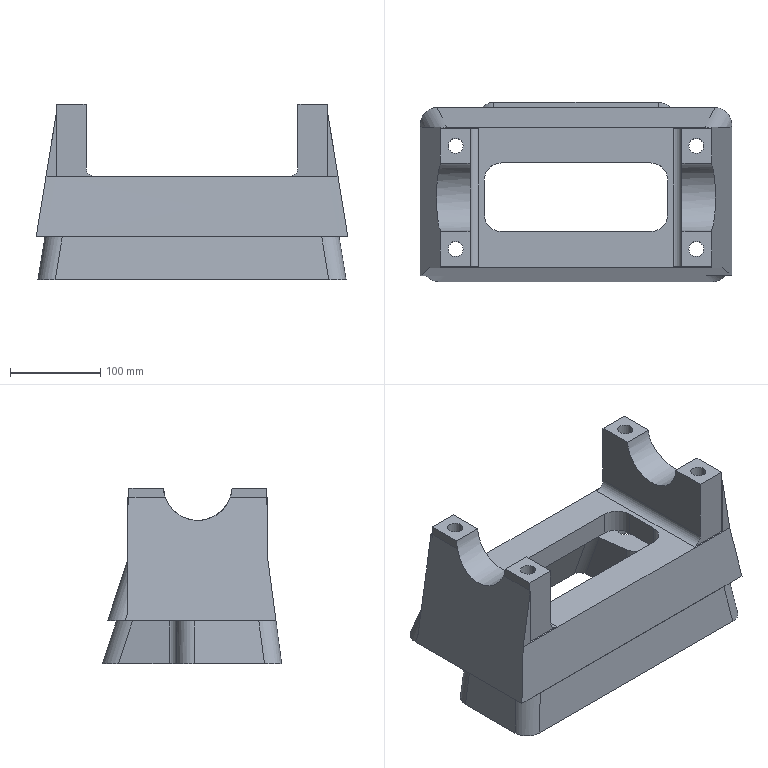Part | SolidWorks | features ICE 7, Fillet 5, Blend 2, Shell 1 | 1 solid | 101 faces | box 345.24 x 198.628 x 194.462 mm | volume 2581916 mm3 | plane 61 | cylinder 38 | spline 2 | commonest cylinder face diameters 16.669 x12 19.304 x10 38.608 x10 38.1 x4 76.2 x2